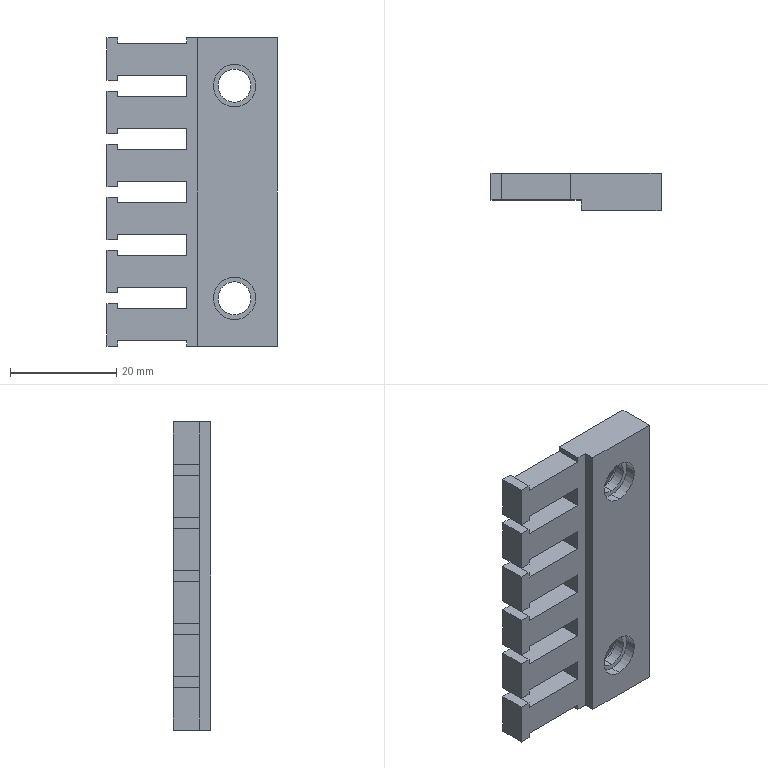Part | SolidWorks | features BaseBody 1 | 1 solid | 76 faces | box 32 x 7 x 58 mm | volume 8749 mm3 | plane 60 | cylinder 12 | cone 4 | commonest cylinder face diameters 8 x8 6.2 x4